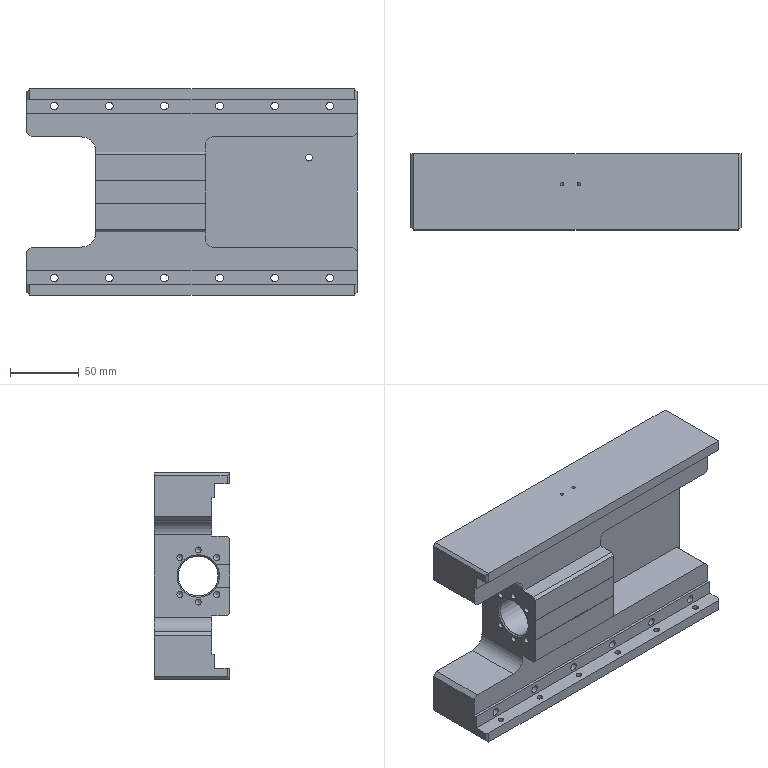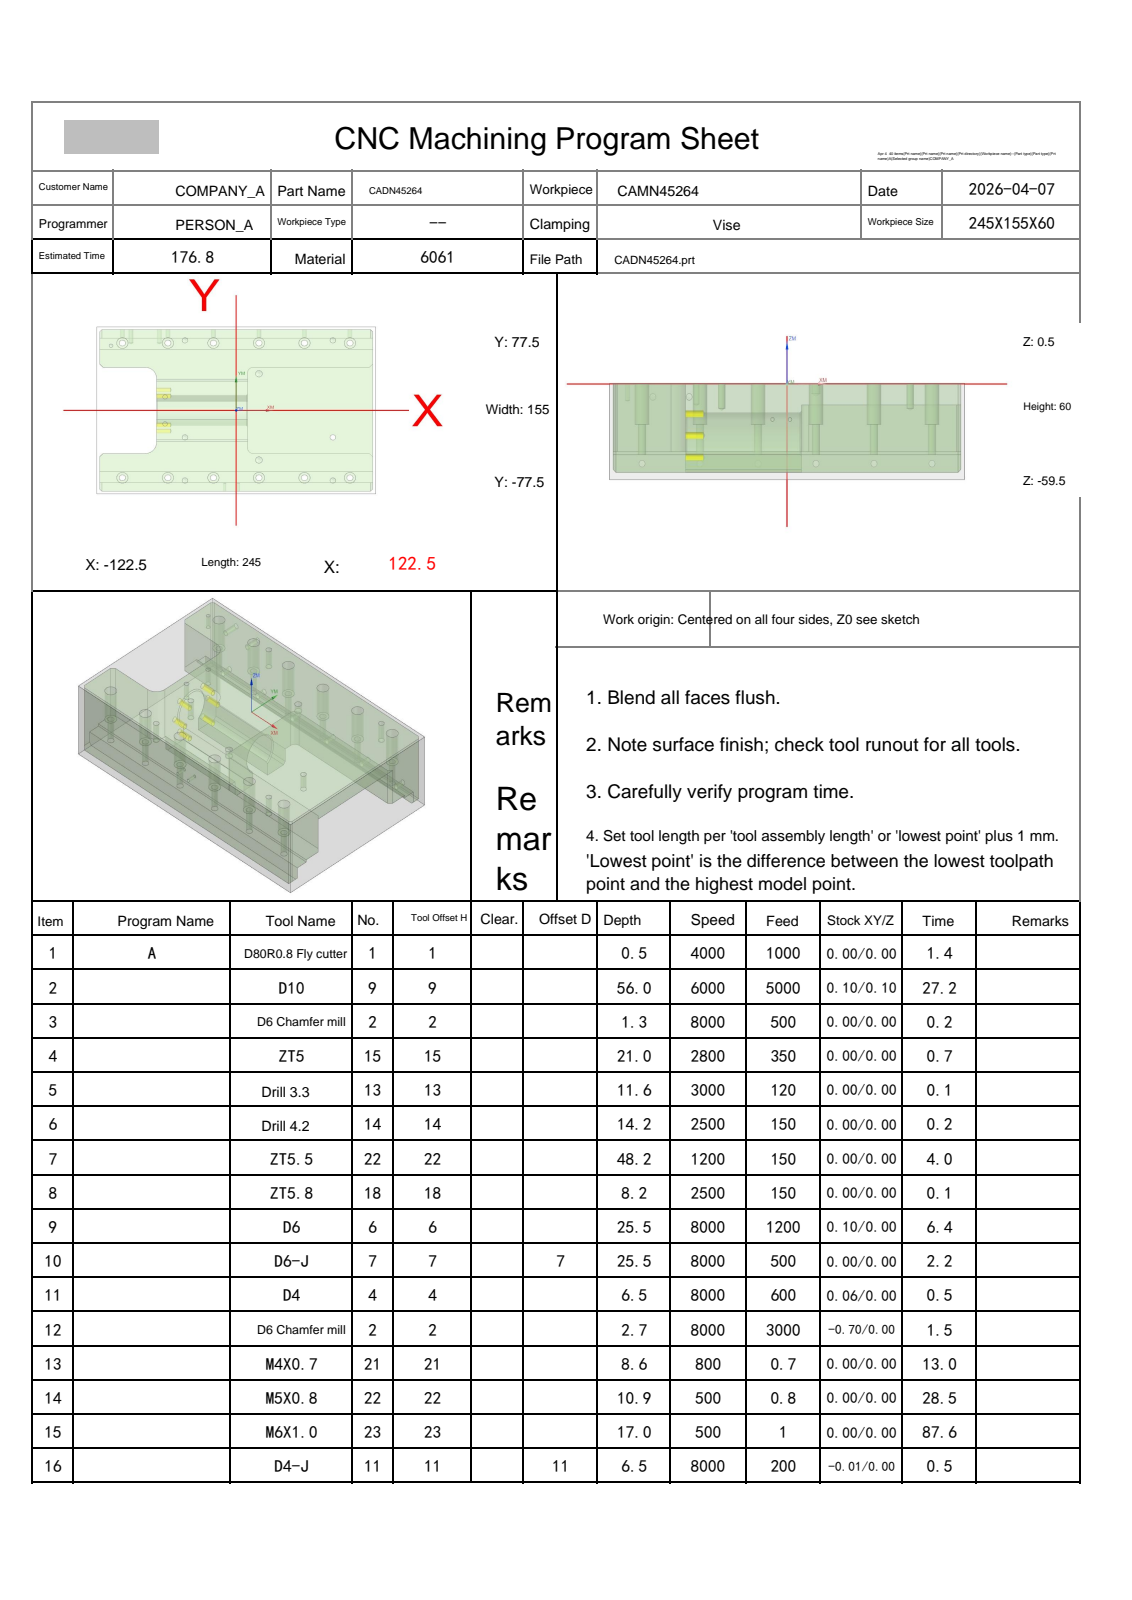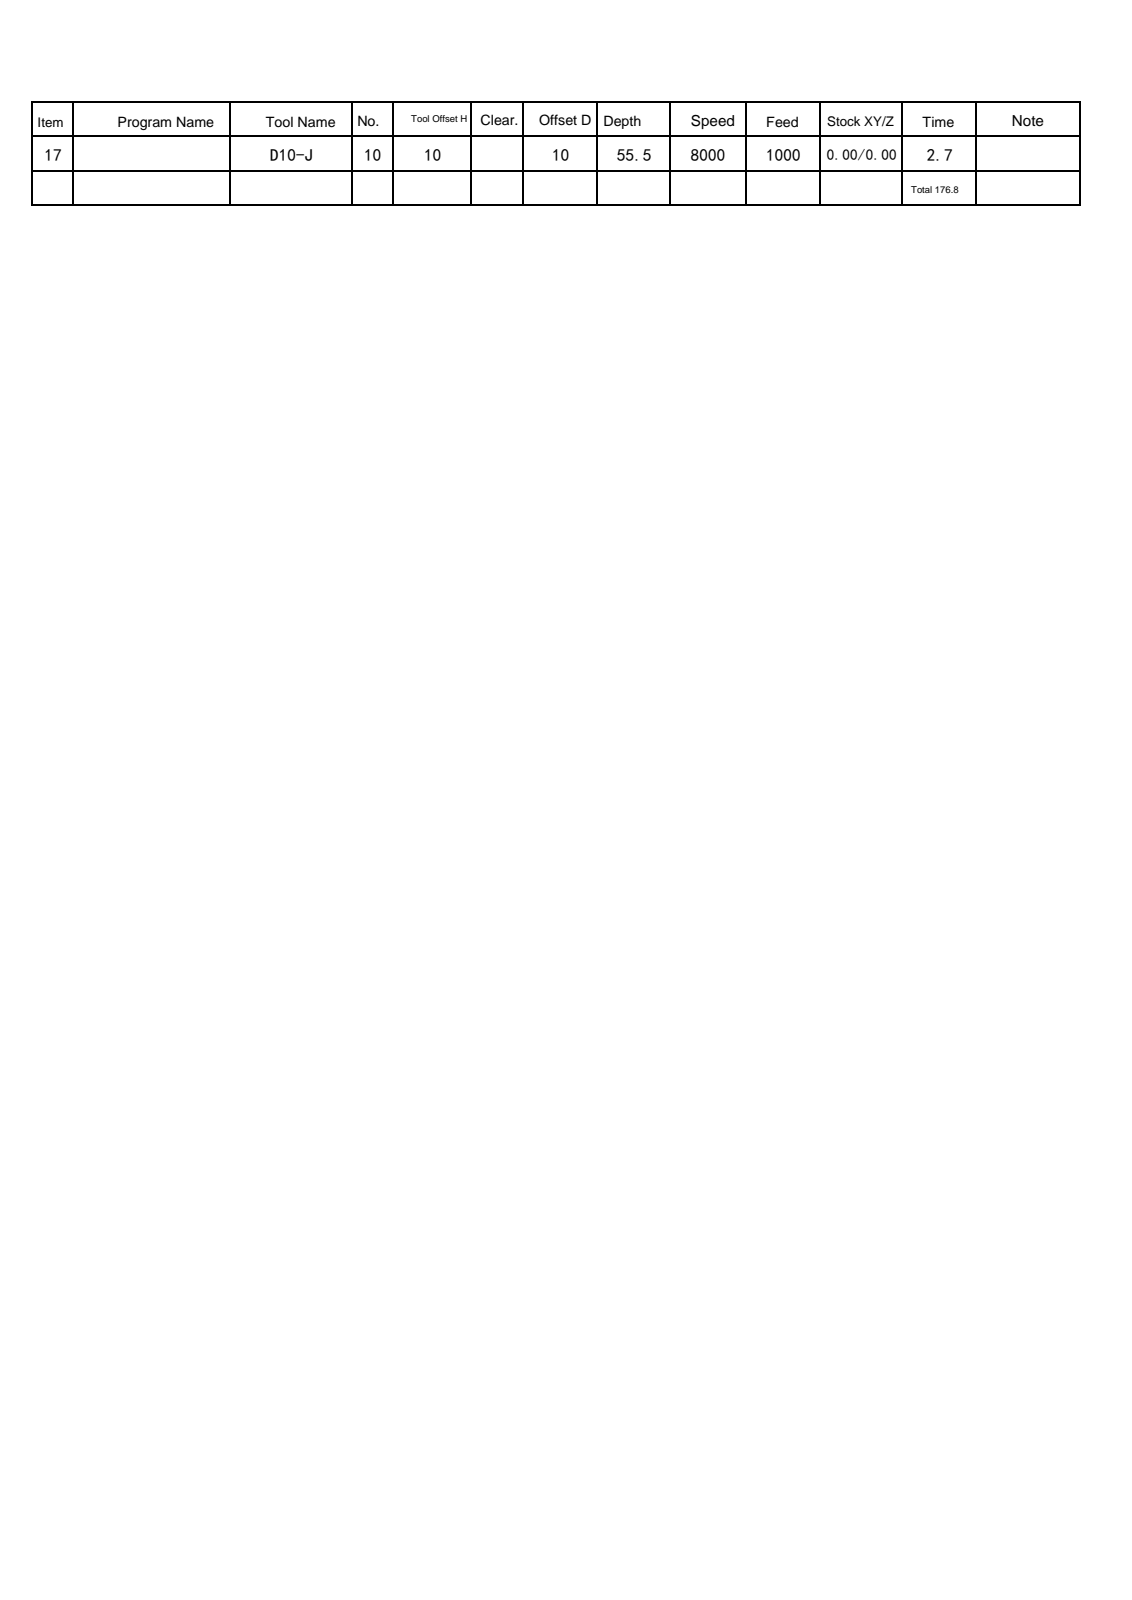NC program | NX | posted by the shop | part box 240 x 55 x 150 mm
Lines 1 to 47 of 12612:
%
O0001
(Machine time: 299.05 MIN)
(===Total Tool:15===)
(T1=D80R0.8 Fly cutter D=80.  R=0.8  D-  H01 Z=-0.   )
(T9=D10     D=10.  R=0.   D-  H09 Z=-55.53)
(T2=D6 Chamfer mill   D=6.   R=0.   D-  H02 Z=-2.2  )
(T15=ZT5    D=5.   DR_a=118 D-  H15 Z=-20.5 )
(T13=Drill 3.3  D=3.3  DR_a=118 D-  H13 Z=-11.09)
(T14=Drill 4.2  D=4.2  DR_a=118 D-  H14 Z=-13.66)
(T22=ZT5.5  D=5.5  DR_a=118 D-  H22 Z=-47.65)
(T18=ZT5.8  D=5.8  DR_a=118 D-  H18 Z=-7.7  )
(T6=D6      D=6.   R=0.   D-  H06 Z=-25.  )
(T7=D6-J    D=6.   R=0.   D7  H07 Z=-25.  )
(T4=D4      D=4.   R=0.   D-  H04 Z=-6.   )
(T21=M4X0.7 D=3.3  DR_a=180 D-  H21 Z=-8.1  )
(T23=M6X1.0 D=5.   DR_a=180 D-  H23 Z=-16.5 )
(T11=D4-J   D=4.   R=0.   D11 H11 Z=-6.   )
(T10=D10-J  D=10.  R=0.   D10 H10 Z=-55.  )
G80 G90 G17 G49 G40
G91 G28 Z0
M01
N1 T01 M06
(D80R0.8 Fly cutter  D=80. R=0.8 H=01 ce=0.00 di=0.00)
G00 G90 G54 X165. Y-69. M03 S4000
G43 H01 Z20.
M08
Z2.
G01 Z0.0 F1000.
X160.
X-160.
Y-23.
X160.
Y23.
X-160.
Y69.
X160.
X165.
Z2.
G00 Z20.
G91 G28 Z0.0
M05
M09
G91 G28 Z0.0
M01